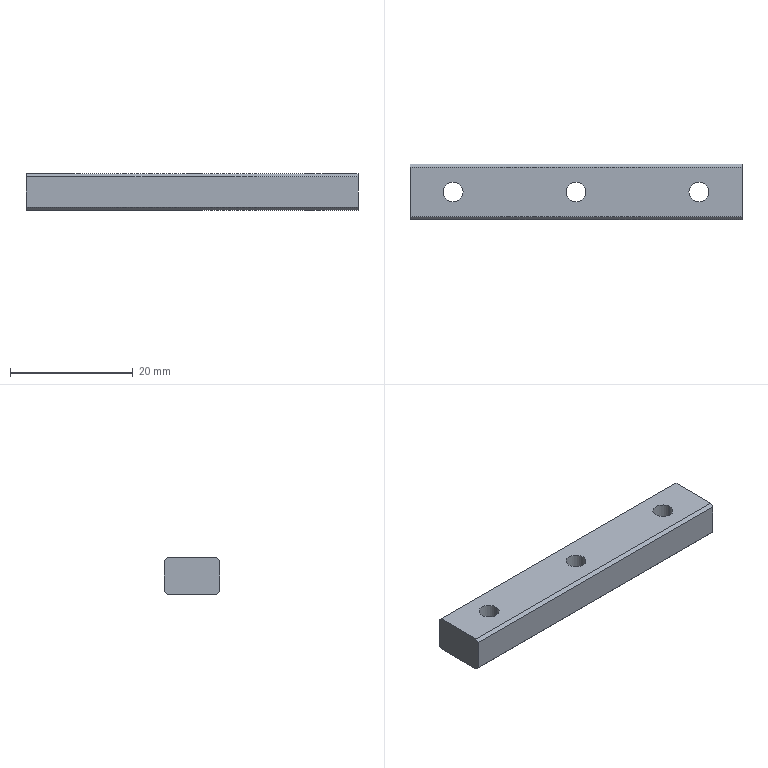Part | SolidWorks | features BaseBody 1 | 1 solid | 16 faces | box 54 x 9 x 6 mm | volume 2740 mm3 | plane 10 | cylinder 6 | commonest cylinder face diameters 3.242 x6
STEP:
#1=CARTESIAN_POINT('',(-9.151,-0.4464,0.));
#2=VERTEX_POINT('',#1);
#3=CARTESIAN_POINT('',(-5.909,-0.4464,0.));
#4=VERTEX_POINT('',#3);
#5=CARTESIAN_POINT('',(-7.53,-0.4464,0.));
#6=DIRECTION('',(0.,0.,1.));
#7=DIRECTION('',(1.,0.,0.));
#8=AXIS2_PLACEMENT_3D('',#5,#6,#7);
#9=CIRCLE('',#8,1.621);
#10=EDGE_CURVE('',#2,#4,#9,.T.);
#11=ORIENTED_EDGE('',*,*,#10,.F.);
#12=CARTESIAN_POINT('',(-9.151,-0.4464,6.));
#13=VERTEX_POINT('',#12);
#14=CARTESIAN_POINT('',(-9.151,-0.4464,-49.073));
#15=DIRECTION('',(0.,0.,1.));
#16=VECTOR('',#15,1000.);
#17=LINE('',#14,#16);
#18=EDGE_CURVE('',#2,#13,#17,.T.);
#19=ORIENTED_EDGE('',*,*,#18,.T.);
#20=CARTESIAN_POINT('',(-5.909,-0.4464,6.));
#21=VERTEX_POINT('',#20);
#22=CARTESIAN_POINT('',(-7.53,-0.4464,6.));
#23=DIRECTION('',(0.,0.,-1.));
#24=DIRECTION('',(1.,0.,0.));
#25=AXIS2_PLACEMENT_3D('',#22,#23,#24);
#26=CIRCLE('',#25,1.621);
#27=EDGE_CURVE('',#21,#13,#26,.T.);
#28=ORIENTED_EDGE('',*,*,#27,.F.);
#29=CARTESIAN_POINT('',(-5.909,-0.4464,-49.073));
#30=DIRECTION('',(0.,0.,1.));
#31=VECTOR('',#30,1000.);
#32=LINE('',#29,#31);
#33=EDGE_CURVE('',#4,#21,#32,.T.);
#34=ORIENTED_EDGE('',*,*,#33,.F.);
#35=EDGE_LOOP('',(#11,#19,#28,#34));
#36=FACE_OUTER_BOUND('',#35,.T.);
#37=CARTESIAN_POINT('',(-7.53,-0.4464,-49.073));
#38=DIRECTION('',(0.,0.,1.));
#39=DIRECTION('',(1.,0.,0.));
#40=AXIS2_PLACEMENT_3D('',#37,#38,#39);
#41=CYLINDRICAL_SURFACE('',#40,1.621);
#42=ADVANCED_FACE('',(#36),#41,.F.);
#43=CARTESIAN_POINT('',(10.849,-0.4464,0.));
#44=VERTEX_POINT('',#43);
#45=CARTESIAN_POINT('',(14.091,-0.4464,0.));
#46=VERTEX_POINT('',#45);
#47=CARTESIAN_POINT('',(12.47,-0.4464,0.));
#48=DIRECTION('',(0.,0.,1.));
#49=DIRECTION('',(1.,0.,0.));
#50=AXIS2_PLACEMENT_3D('',#47,#48,#49);
#51=CIRCLE('',#50,1.621);
#52=EDGE_CURVE('',#44,#46,#51,.T.);
#53=ORIENTED_EDGE('',*,*,#52,.F.);
#54=CARTESIAN_POINT('',(10.849,-0.4464,6.));
#55=VERTEX_POINT('',#54);
#56=CARTESIAN_POINT('',(10.849,-0.4464,-49.073));
#57=DIRECTION('',(0.,0.,1.));
#58=VECTOR('',#57,1000.);
#59=LINE('',#56,#58);
#60=EDGE_CURVE('',#44,#55,#59,.T.);
#61=ORIENTED_EDGE('',*,*,#60,.T.);
#62=CARTESIAN_POINT('',(14.091,-0.4464,6.));
#63=VERTEX_POINT('',#62);
#64=CARTESIAN_POINT('',(12.47,-0.4464,6.));
#65=DIRECTION('',(0.,0.,-1.));
#66=DIRECTION('',(1.,0.,0.));
#67=AXIS2_PLACEMENT_3D('',#64,#65,#66);
#68=CIRCLE('',#67,1.621);
#69=EDGE_CURVE('',#63,#55,#68,.T.);
#70=ORIENTED_EDGE('',*,*,#69,.F.);
#71=CARTESIAN_POINT('',(14.091,-0.4464,-49.073));
#72=DIRECTION('',(0.,0.,1.));
#73=VECTOR('',#72,1000.);
#74=LINE('',#71,#73);
#75=EDGE_CURVE('',#46,#63,#74,.T.);
#76=ORIENTED_EDGE('',*,*,#75,.F.);
#77=EDGE_LOOP('',(#53,#61,#70,#76));
#78=FACE_OUTER_BOUND('',#77,.T.);
#79=CARTESIAN_POINT('',(12.47,-0.4464,-49.073));
#80=DIRECTION('',(0.,0.,1.));
#81=DIRECTION('',(1.,0.,0.));
#82=AXIS2_PLACEMENT_3D('',#79,#80,#81);
#83=CYLINDRICAL_SURFACE('',#82,1.621);
#84=ADVANCED_FACE('',(#78),#83,.F.);
#85=CARTESIAN_POINT('',(30.849,-0.4464,0.));
#86=VERTEX_POINT('',#85);
#87=CARTESIAN_POINT('',(34.091,-0.4464,0.));
#88=VERTEX_POINT('',#87);
#89=CARTESIAN_POINT('',(32.47,-0.4464,0.));
#90=DIRECTION('',(0.,0.,1.));
#91=DIRECTION('',(1.,0.,0.));
#92=AXIS2_PLACEMENT_3D('',#89,#90,#91);
#93=CIRCLE('',#92,1.621);
#94=EDGE_CURVE('',#86,#88,#93,.T.);
#95=ORIENTED_EDGE('',*,*,#94,.F.);
#96=CARTESIAN_POINT('',(30.849,-0.4464,6.));
#97=VERTEX_POINT('',#96);
#98=CARTESIAN_POINT('',(30.849,-0.4464,-49.073));
#99=DIRECTION('',(0.,0.,1.));
#100=VECTOR('',#99,1000.);
#101=LINE('',#98,#100);
#102=EDGE_CURVE('',#86,#97,#101,.T.);
#103=ORIENTED_EDGE('',*,*,#102,.T.);
#104=CARTESIAN_POINT('',(34.091,-0.4464,6.));
#105=VERTEX_POINT('',#104);
#106=CARTESIAN_POINT('',(32.47,-0.4464,6.));
#107=DIRECTION('',(0.,0.,-1.));
#108=DIRECTION('',(1.,0.,0.));
#109=AXIS2_PLACEMENT_3D('',#106,#107,#108);
#110=CIRCLE('',#109,1.621);
#111=EDGE_CURVE('',#105,#97,#110,.T.);
#112=ORIENTED_EDGE('',*,*,#111,.F.);
#113=CARTESIAN_POINT('',(34.091,-0.4464,-49.073));
#114=DIRECTION('',(0.,0.,1.));
#115=VECTOR('',#114,1000.);
#116=LINE('',#113,#115);
#117=EDGE_CURVE('',#88,#105,#116,.T.);
#118=ORIENTED_EDGE('',*,*,#117,.F.);
#119=EDGE_LOOP('',(#95,#103,#112,#118));
#120=FACE_OUTER_BOUND('',#119,.T.);
#121=CARTESIAN_POINT('',(32.47,-0.4464,-49.073));
#122=DIRECTION('',(0.,0.,1.));
#123=DIRECTION('',(1.,0.,0.));
#124=AXIS2_PLACEMENT_3D('',#121,#122,#123);
#125=CYLINDRICAL_SURFACE('',#124,1.621);
#126=ADVANCED_FACE('',(#120),#125,.F.);
#127=ORIENTED_EDGE('',*,*,#27,.T.);
#128=CARTESIAN_POINT('',(-7.53,-0.4464,6.));
#129=DIRECTION('',(0.,0.,-1.));
#130=DIRECTION('',(1.,0.,0.));
#131=AXIS2_PLACEMENT_3D('',#128,#129,#130);
#132=CIRCLE('',#131,1.621);
#133=EDGE_CURVE('',#13,#21,#132,.T.);
#134=ORIENTED_EDGE('',*,*,#133,.T.);
#135=EDGE_LOOP('',(#127,#134));
#136=FACE_BOUND('',#135,.T.);
#137=ORIENTED_EDGE('',*,*,#69,.T.);
#138=CARTESIAN_POINT('',(12.47,-0.4464,6.));
#139=DIRECTION('',(0.,0.,-1.));
#140=DIRECTION('',(1.,0.,0.));
#141=AXIS2_PLACEMENT_3D('',#138,#139,#140);
#142=CIRCLE('',#141,1.621);
#143=EDGE_CURVE('',#55,#63,#142,.T.);
#144=ORIENTED_EDGE('',*,*,#143,.T.);
#145=EDGE_LOOP('',(#137,#144));
#146=FACE_BOUND('',#145,.T.);
#147=ORIENTED_EDGE('',*,*,#111,.T.);
#148=CARTESIAN_POINT('',(32.47,-0.4464,6.));
#149=DIRECTION('',(0.,0.,-1.));
#150=DIRECTION('',(1.,0.,0.));
#151=AXIS2_PLACEMENT_3D('',#148,#149,#150);
#152=CIRCLE('',#151,1.621);
#153=EDGE_CURVE('',#97,#105,#152,.T.);
#154=ORIENTED_EDGE('',*,*,#153,.T.);
#155=EDGE_LOOP('',(#147,#154));
#156=FACE_BOUND('',#155,.T.);
#157=CARTESIAN_POINT('',(39.47,3.554,6.));
#158=VERTEX_POINT('',#157);
#159=CARTESIAN_POINT('',(-14.53,3.554,6.));
#160=VERTEX_POINT('',#159);
#161=CARTESIAN_POINT('',(12.47,3.554,6.));
#162=DIRECTION('',(-1.,0.,0.));
#163=VECTOR('',#162,1000.);
#164=LINE('',#161,#163);
#165=EDGE_CURVE('',#158,#160,#164,.T.);
#166=ORIENTED_EDGE('',*,*,#165,.T.);
#167=CARTESIAN_POINT('',(-14.53,-4.446,6.));
#168=VERTEX_POINT('',#167);
#169=CARTESIAN_POINT('',(-14.53,-0.4464,6.));
#170=DIRECTION('',(0.,-1.,0.));
#171=VECTOR('',#170,1000.);
#172=LINE('',#169,#171);
#173=EDGE_CURVE('',#160,#168,#172,.T.);
#174=ORIENTED_EDGE('',*,*,#173,.T.);
#175=CARTESIAN_POINT('',(39.47,-4.446,6.));
#176=VERTEX_POINT('',#175);
#177=CARTESIAN_POINT('',(12.47,-4.446,6.));
#178=DIRECTION('',(1.,0.,0.));
#179=VECTOR('',#178,1000.);
#180=LINE('',#177,#179);
#181=EDGE_CURVE('',#168,#176,#180,.T.);
#182=ORIENTED_EDGE('',*,*,#181,.T.);
#183=CARTESIAN_POINT('',(39.47,-0.4464,6.));
#184=DIRECTION('',(0.,1.,0.));
#185=VECTOR('',#184,1000.);
#186=LINE('',#183,#185);
#187=EDGE_CURVE('',#176,#158,#186,.T.);
#188=ORIENTED_EDGE('',*,*,#187,.T.);
#189=EDGE_LOOP('',(#166,#174,#182,#188));
#190=FACE_OUTER_BOUND('',#189,.T.);
#191=CARTESIAN_POINT('',(12.47,-0.4464,6.));
#192=DIRECTION('',(0.,0.,1.));
#193=DIRECTION('',(1.,0.,0.));
#194=AXIS2_PLACEMENT_3D('',#191,#192,#193);
#195=PLANE('',#194);
#196=ADVANCED_FACE('',(#136,#146,#156,#190),#195,.T.);
#197=ORIENTED_EDGE('',*,*,#18,.F.);
#198=CARTESIAN_POINT('',(-7.53,-0.4464,0.));
#199=DIRECTION('',(0.,0.,1.));
#200=DIRECTION('',(1.,0.,0.));
#201=AXIS2_PLACEMENT_3D('',#198,#199,#200);
#202=CIRCLE('',#201,1.621);
#203=EDGE_CURVE('',#4,#2,#202,.T.);
#204=ORIENTED_EDGE('',*,*,#203,.F.);
#205=ORIENTED_EDGE('',*,*,#33,.T.);
#206=ORIENTED_EDGE('',*,*,#133,.F.);
#207=EDGE_LOOP('',(#197,#204,#205,#206));
#208=FACE_OUTER_BOUND('',#207,.T.);
#209=CARTESIAN_POINT('',(-7.53,-0.4464,-49.073));
#210=DIRECTION('',(0.,0.,1.));
#211=DIRECTION('',(1.,0.,0.));
#212=AXIS2_PLACEMENT_3D('',#209,#210,#211);
#213=CYLINDRICAL_SURFACE('',#212,1.621);
#214=ADVANCED_FACE('',(#208),#213,.F.);
#215=ORIENTED_EDGE('',*,*,#60,.F.);
#216=CARTESIAN_POINT('',(12.47,-0.4464,0.));
#217=DIRECTION('',(0.,0.,1.));
#218=DIRECTION('',(1.,0.,0.));
#219=AXIS2_PLACEMENT_3D('',#216,#217,#218);
#220=CIRCLE('',#219,1.621);
#221=EDGE_CURVE('',#46,#44,#220,.T.);
#222=ORIENTED_EDGE('',*,*,#221,.F.);
#223=ORIENTED_EDGE('',*,*,#75,.T.);
#224=ORIENTED_EDGE('',*,*,#143,.F.);
#225=EDGE_LOOP('',(#215,#222,#223,#224));
#226=FACE_OUTER_BOUND('',#225,.T.);
#227=CARTESIAN_POINT('',(12.47,-0.4464,-49.073));
#228=DIRECTION('',(0.,0.,1.));
#229=DIRECTION('',(1.,0.,0.));
#230=AXIS2_PLACEMENT_3D('',#227,#228,#229);
#231=CYLINDRICAL_SURFACE('',#230,1.621);
#232=ADVANCED_FACE('',(#226),#231,.F.);
#233=ORIENTED_EDGE('',*,*,#102,.F.);
#234=CARTESIAN_POINT('',(32.47,-0.4464,0.));
#235=DIRECTION('',(0.,0.,1.));
#236=DIRECTION('',(1.,0.,0.));
#237=AXIS2_PLACEMENT_3D('',#234,#235,#236);
#238=CIRCLE('',#237,1.621);
#239=EDGE_CURVE('',#88,#86,#238,.T.);
#240=ORIENTED_EDGE('',*,*,#239,.F.);
#241=ORIENTED_EDGE('',*,*,#117,.T.);
#242=ORIENTED_EDGE('',*,*,#153,.F.);
#243=EDGE_LOOP('',(#233,#240,#241,#242));
#244=FACE_OUTER_BOUND('',#243,.T.);
#245=CARTESIAN_POINT('',(32.47,-0.4464,-49.073));
#246=DIRECTION('',(0.,0.,1.));
#247=DIRECTION('',(1.,0.,0.));
#248=AXIS2_PLACEMENT_3D('',#245,#246,#247);
#249=CYLINDRICAL_SURFACE('',#248,1.621);
#250=ADVANCED_FACE('',(#244),#249,.F.);
#251=CARTESIAN_POINT('',(-14.53,4.054,5.5));
#252=VERTEX_POINT('',#251);
#253=CARTESIAN_POINT('',(-14.53,3.554,6.));
#254=DIRECTION('',(0.,0.7071,-0.7071));
#255=VECTOR('',#254,1000.);
#256=LINE('',#253,#255);
#257=EDGE_CURVE('',#160,#252,#256,.T.);
#258=ORIENTED_EDGE('',*,*,#257,.T.);
#259=CARTESIAN_POINT('',(-14.53,4.054,0.5));
#260=VERTEX_POINT('',#259);
#261=CARTESIAN_POINT('',(-14.53,4.054,0.));
#262=DIRECTION('',(0.,0.,-1.));
#263=VECTOR('',#262,1000.);
#264=LINE('',#261,#263);
#265=EDGE_CURVE('',#252,#260,#264,.T.);
#266=ORIENTED_EDGE('',*,*,#265,.T.);
#267=CARTESIAN_POINT('',(-14.53,3.554,0.));
#268=VERTEX_POINT('',#267);
#269=CARTESIAN_POINT('',(-14.53,3.804,0.25));
#270=DIRECTION('',(0.,0.7071,0.7071));
#271=VECTOR('',#270,1000.);
#272=LINE('',#269,#271);
#273=EDGE_CURVE('',#268,#260,#272,.T.);
#274=ORIENTED_EDGE('',*,*,#273,.F.);
#275=CARTESIAN_POINT('',(-14.53,-4.446,0.));
#276=VERTEX_POINT('',#275);
#277=CARTESIAN_POINT('',(-14.53,-4.946,0.));
#278=DIRECTION('',(0.,-1.,0.));
#279=VECTOR('',#278,1000.);
#280=LINE('',#277,#279);
#281=EDGE_CURVE('',#268,#276,#280,.T.);
#282=ORIENTED_EDGE('',*,*,#281,.T.);
#283=CARTESIAN_POINT('',(-14.53,-4.946,0.5));
#284=VERTEX_POINT('',#283);
#285=CARTESIAN_POINT('',(-14.53,-4.696,0.25));
#286=DIRECTION('',(0.,0.7071,-0.7071));
#287=VECTOR('',#286,1000.);
#288=LINE('',#285,#287);
#289=EDGE_CURVE('',#284,#276,#288,.T.);
#290=ORIENTED_EDGE('',*,*,#289,.F.);
#291=CARTESIAN_POINT('',(-14.53,-4.946,5.5));
#292=VERTEX_POINT('',#291);
#293=CARTESIAN_POINT('',(-14.53,-4.946,0.));
#294=DIRECTION('',(0.,0.,1.));
#295=VECTOR('',#294,1000.);
#296=LINE('',#293,#295);
#297=EDGE_CURVE('',#284,#292,#296,.T.);
#298=ORIENTED_EDGE('',*,*,#297,.T.);
#299=CARTESIAN_POINT('',(-14.53,-4.946,5.5));
#300=DIRECTION('',(0.,0.7071,0.7071));
#301=VECTOR('',#300,1000.);
#302=LINE('',#299,#301);
#303=EDGE_CURVE('',#292,#168,#302,.T.);
#304=ORIENTED_EDGE('',*,*,#303,.T.);
#305=ORIENTED_EDGE('',*,*,#173,.F.);
#306=EDGE_LOOP('',(#258,#266,#274,#282,#290,#298,#304,#305));
#307=FACE_OUTER_BOUND('',#306,.T.);
#308=CARTESIAN_POINT('',(-14.53,-4.946,0.));
#309=DIRECTION('',(-1.,0.,0.));
#310=DIRECTION('',(0.,0.,1.));
#311=AXIS2_PLACEMENT_3D('',#308,#309,#310);
#312=PLANE('',#311);
#313=ADVANCED_FACE('',(#307),#312,.T.);
#314=ORIENTED_EDGE('',*,*,#257,.F.);
#315=ORIENTED_EDGE('',*,*,#165,.F.);
#316=CARTESIAN_POINT('',(39.47,4.054,5.5));
#317=VERTEX_POINT('',#316);
#318=CARTESIAN_POINT('',(39.47,3.804,5.75));
#319=DIRECTION('',(0.,0.7071,-0.7071));
#320=VECTOR('',#319,1000.);
#321=LINE('',#318,#320);
#322=EDGE_CURVE('',#158,#317,#321,.T.);
#323=ORIENTED_EDGE('',*,*,#322,.T.);
#324=CARTESIAN_POINT('',(-1.03,4.054,5.5));
#325=DIRECTION('',(-1.,0.,0.));
#326=VECTOR('',#325,1000.);
#327=LINE('',#324,#326);
#328=EDGE_CURVE('',#317,#252,#327,.T.);
#329=ORIENTED_EDGE('',*,*,#328,.T.);
#330=EDGE_LOOP('',(#314,#315,#323,#329));
#331=FACE_OUTER_BOUND('',#330,.T.);
#332=CARTESIAN_POINT('',(-1.03,3.804,5.75));
#333=DIRECTION('',(0.,0.7071,0.7071));
#334=DIRECTION('',(0.,-0.7071,0.7071));
#335=AXIS2_PLACEMENT_3D('',#332,#333,#334);
#336=PLANE('',#335);
#337=ADVANCED_FACE('',(#331),#336,.T.);
#338=CARTESIAN_POINT('',(39.47,-4.446,0.));
#339=VERTEX_POINT('',#338);
#340=CARTESIAN_POINT('',(39.47,-4.946,0.5));
#341=VERTEX_POINT('',#340);
#342=CARTESIAN_POINT('',(39.47,-4.696,0.25));
#343=DIRECTION('',(0.,-0.7071,0.7071));
#344=VECTOR('',#343,1000.);
#345=LINE('',#342,#344);
#346=EDGE_CURVE('',#339,#341,#345,.T.);
#347=ORIENTED_EDGE('',*,*,#346,.F.);
#348=CARTESIAN_POINT('',(39.47,3.554,0.));
#349=VERTEX_POINT('',#348);
#350=CARTESIAN_POINT('',(39.47,4.054,0.));
#351=DIRECTION('',(0.,1.,0.));
#352=VECTOR('',#351,1000.);
#353=LINE('',#350,#352);
#354=EDGE_CURVE('',#339,#349,#353,.T.);
#355=ORIENTED_EDGE('',*,*,#354,.T.);
#356=CARTESIAN_POINT('',(39.47,4.054,0.5));
#357=VERTEX_POINT('',#356);
#358=CARTESIAN_POINT('',(39.47,3.804,0.25));
#359=DIRECTION('',(0.,-0.7071,-0.7071));
#360=VECTOR('',#359,1000.);
#361=LINE('',#358,#360);
#362=EDGE_CURVE('',#357,#349,#361,.T.);
#363=ORIENTED_EDGE('',*,*,#362,.F.);
#364=CARTESIAN_POINT('',(39.47,4.054,0.));
#365=DIRECTION('',(0.,0.,1.));
#366=VECTOR('',#365,1000.);
#367=LINE('',#364,#366);
#368=EDGE_CURVE('',#357,#317,#367,.T.);
#369=ORIENTED_EDGE('',*,*,#368,.T.);
#370=ORIENTED_EDGE('',*,*,#322,.F.);
#371=ORIENTED_EDGE('',*,*,#187,.F.);
#372=CARTESIAN_POINT('',(39.47,-4.946,5.5));
#373=VERTEX_POINT('',#372);
#374=CARTESIAN_POINT('',(39.47,-4.446,6.));
#375=DIRECTION('',(0.,-0.7071,-0.7071));
#376=VECTOR('',#375,1000.);
#377=LINE('',#374,#376);
#378=EDGE_CURVE('',#176,#373,#377,.T.);
#379=ORIENTED_EDGE('',*,*,#378,.T.);
#380=CARTESIAN_POINT('',(39.47,-4.946,0.));
#381=DIRECTION('',(0.,0.,-1.));
#382=VECTOR('',#381,1000.);
#383=LINE('',#380,#382);
#384=EDGE_CURVE('',#373,#341,#383,.T.);
#385=ORIENTED_EDGE('',*,*,#384,.T.);
#386=EDGE_LOOP('',(#347,#355,#363,#369,#370,#371,#379,#385));
#387=FACE_OUTER_BOUND('',#386,.T.);
#388=CARTESIAN_POINT('',(39.47,4.054,0.));
#389=DIRECTION('',(1.,0.,0.));
#390=DIRECTION('',(0.,0.,-1.));
#391=AXIS2_PLACEMENT_3D('',#388,#389,#390);
#392=PLANE('',#391);
#393=ADVANCED_FACE('',(#387),#392,.T.);
#394=ORIENTED_EDGE('',*,*,#378,.F.);
#395=ORIENTED_EDGE('',*,*,#181,.F.);
#396=ORIENTED_EDGE('',*,*,#303,.F.);
#397=CARTESIAN_POINT('',(25.97,-4.946,5.5));
#398=DIRECTION('',(1.,0.,0.));
#399=VECTOR('',#398,1000.);
#400=LINE('',#397,#399);
#401=EDGE_CURVE('',#292,#373,#400,.T.);
#402=ORIENTED_EDGE('',*,*,#401,.T.);
#403=EDGE_LOOP('',(#394,#395,#396,#402));
#404=FACE_OUTER_BOUND('',#403,.T.);
#405=CARTESIAN_POINT('',(25.97,-4.696,5.75));
#406=DIRECTION('',(0.,-0.7071,0.7071));
#407=DIRECTION('',(0.,-0.7071,-0.7071));
#408=AXIS2_PLACEMENT_3D('',#405,#406,#407);
#409=PLANE('',#408);
#410=ADVANCED_FACE('',(#404),#409,.T.);
#411=ORIENTED_EDGE('',*,*,#203,.T.);
#412=ORIENTED_EDGE('',*,*,#10,.T.);
#413=EDGE_LOOP('',(#411,#412));
#414=FACE_BOUND('',#413,.T.);
#415=ORIENTED_EDGE('',*,*,#221,.T.);
#416=ORIENTED_EDGE('',*,*,#52,.T.);
#417=EDGE_LOOP('',(#415,#416));
#418=FACE_BOUND('',#417,.T.);
#419=ORIENTED_EDGE('',*,*,#239,.T.);
#420=ORIENTED_EDGE('',*,*,#94,.T.);
#421=EDGE_LOOP('',(#419,#420));
#422=FACE_BOUND('',#421,.T.);
#423=ORIENTED_EDGE('',*,*,#354,.F.);
#424=CARTESIAN_POINT('',(12.47,-4.446,0.));
#425=DIRECTION('',(1.,0.,0.));
#426=VECTOR('',#425,1000.);
#427=LINE('',#424,#426);
#428=EDGE_CURVE('',#276,#339,#427,.T.);
#429=ORIENTED_EDGE('',*,*,#428,.F.);
#430=ORIENTED_EDGE('',*,*,#281,.F.);
#431=CARTESIAN_POINT('',(12.47,3.554,0.));
#432=DIRECTION('',(-1.,0.,0.));
#433=VECTOR('',#432,1000.);
#434=LINE('',#431,#433);
#435=EDGE_CURVE('',#349,#268,#434,.T.);
#436=ORIENTED_EDGE('',*,*,#435,.F.);
#437=EDGE_LOOP('',(#423,#429,#430,#436));
#438=FACE_OUTER_BOUND('',#437,.T.);
#439=CARTESIAN_POINT('',(12.47,-0.4464,0.));
#440=DIRECTION('',(0.,0.,1.));
#441=DIRECTION('',(1.,0.,0.));
#442=AXIS2_PLACEMENT_3D('',#439,#440,#441);
#443=PLANE('',#442);
#444=ADVANCED_FACE('',(#414,#418,#422,#438),#443,.F.);
#445=ORIENTED_EDGE('',*,*,#328,.F.);
#446=ORIENTED_EDGE('',*,*,#368,.F.);
#447=CARTESIAN_POINT('',(-14.53,4.054,0.5));
#448=DIRECTION('',(-1.,0.,0.));
#449=VECTOR('',#448,1000.);
#450=LINE('',#447,#449);
#451=EDGE_CURVE('',#357,#260,#450,.T.);
#452=ORIENTED_EDGE('',*,*,#451,.T.);
#453=ORIENTED_EDGE('',*,*,#265,.F.);
#454=EDGE_LOOP('',(#445,#446,#452,#453));
#455=FACE_OUTER_BOUND('',#454,.T.);
#456=CARTESIAN_POINT('',(-14.53,4.054,0.));
#457=DIRECTION('',(0.,1.,0.));
#458=DIRECTION('',(0.,0.,1.));
#459=AXIS2_PLACEMENT_3D('',#456,#457,#458);
#460=PLANE('',#459);
#461=ADVANCED_FACE('',(#455),#460,.T.);
#462=ORIENTED_EDGE('',*,*,#401,.F.);
#463=ORIENTED_EDGE('',*,*,#297,.F.);
#464=CARTESIAN_POINT('',(39.47,-4.946,0.5));
#465=DIRECTION('',(1.,0.,0.));
#466=VECTOR('',#465,1000.);
#467=LINE('',#464,#466);
#468=EDGE_CURVE('',#284,#341,#467,.T.);
#469=ORIENTED_EDGE('',*,*,#468,.T.);
#470=ORIENTED_EDGE('',*,*,#384,.F.);
#471=EDGE_LOOP('',(#462,#463,#469,#470));
#472=FACE_OUTER_BOUND('',#471,.T.);
#473=CARTESIAN_POINT('',(39.47,-4.946,0.));
#474=DIRECTION('',(0.,-1.,0.));
#475=DIRECTION('',(0.,0.,-1.));
#476=AXIS2_PLACEMENT_3D('',#473,#474,#475);
#477=PLANE('',#476);
#478=ADVANCED_FACE('',(#472),#477,.T.);
#479=ORIENTED_EDGE('',*,*,#273,.T.);
#480=ORIENTED_EDGE('',*,*,#451,.F.);
#481=ORIENTED_EDGE('',*,*,#362,.T.);
#482=ORIENTED_EDGE('',*,*,#435,.T.);
#483=EDGE_LOOP('',(#479,#480,#481,#482));
#484=FACE_OUTER_BOUND('',#483,.T.);
#485=CARTESIAN_POINT('',(-1.03,3.804,0.25));
#486=DIRECTION('',(0.,0.7071,-0.7071));
#487=DIRECTION('',(0.,0.7071,0.7071));
#488=AXIS2_PLACEMENT_3D('',#485,#486,#487);
#489=PLANE('',#488);
#490=ADVANCED_FACE('',(#484),#489,.T.);
#491=ORIENTED_EDGE('',*,*,#346,.T.);
#492=ORIENTED_EDGE('',*,*,#468,.F.);
#493=ORIENTED_EDGE('',*,*,#289,.T.);
#494=ORIENTED_EDGE('',*,*,#428,.T.);
#495=EDGE_LOOP('',(#491,#492,#493,#494));
#496=FACE_OUTER_BOUND('',#495,.T.);
#497=CARTESIAN_POINT('',(25.97,-4.696,0.25));
#498=DIRECTION('',(0.,-0.7071,-0.7071));
#499=DIRECTION('',(0.,0.7071,-0.7071));
#500=AXIS2_PLACEMENT_3D('',#497,#498,#499);
#501=PLANE('',#500);
#502=ADVANCED_FACE('',(#496),#501,.T.);
#503=CLOSED_SHELL('',(#42,#84,#126,#196,#214,#232,#250,#313,#337,#393,#410,#444,#461,#478,#490,#502));
#504=MANIFOLD_SOLID_BREP('',#503);
#505=CARTESIAN_POINT('',(0.,0.,0.));
#506=DIRECTION('',(0.,0.,1.));
#507=DIRECTION('',(1.,0.,0.));
#508=AXIS2_PLACEMENT_3D('',#505,#506,#507);
#509=(LENGTH_UNIT()NAMED_UNIT(*)SI_UNIT(.MILLI.,.METRE.));
#510=UNCERTAINTY_MEASURE_WITH_UNIT(LENGTH_MEASURE(0.00001),#509,'','');
#511=(NAMED_UNIT(*)PLANE_ANGLE_UNIT()SI_UNIT($,.RADIAN.));
#512=(NAMED_UNIT(*)SI_UNIT($,.STERADIAN.)SOLID_ANGLE_UNIT());
#513=(GEOMETRIC_REPRESENTATION_CONTEXT(3)GLOBAL_UNCERTAINTY_ASSIGNED_CONTEXT((#510))GLOBAL_UNIT_ASSIGNED_CONTEXT((#509,#511,#512))REPRESENTATION_CONTEXT('',''));
#514=ADVANCED_BREP_SHAPE_REPRESENTATION('',(#504,#508),#513);